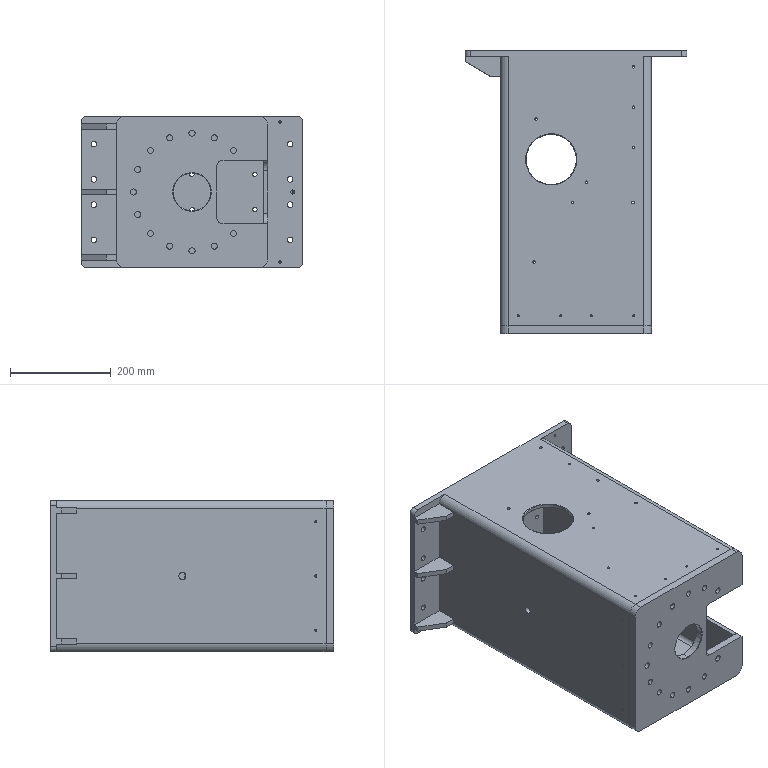Part | SolidWorks | features HoleWzd 11, ICE 7, Chamfer 3, Fillet 3, Cut 2, LPattern 2, MirrorPattern 1, MoveFace 1, WeldMemberFeat 1, WeldmentFeature 1 | 2 solids | 241 faces | box 440 x 562 x 300 mm | volume 7106241 mm3 | cylinder 176 | plane 45 | cone 20 | commonest cylinder face diameters 5 x48 4.2 x38 12 x26 11 x16 8.5 x12 32 x8